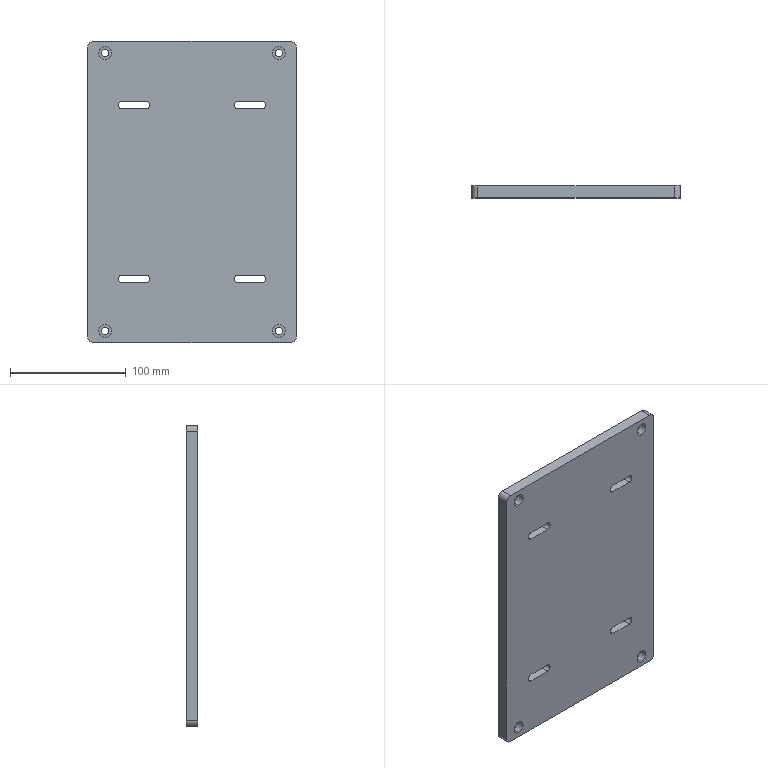Part | STEP file | 0-19-12 Mounting connecting plate | 1 solid | 46 faces | box 180 x 10 x 260 mm | volume 458114 mm3 | cylinder 28 | plane 18 | commonest cylinder face diameters 6.6 x16 11 x8 10 x4